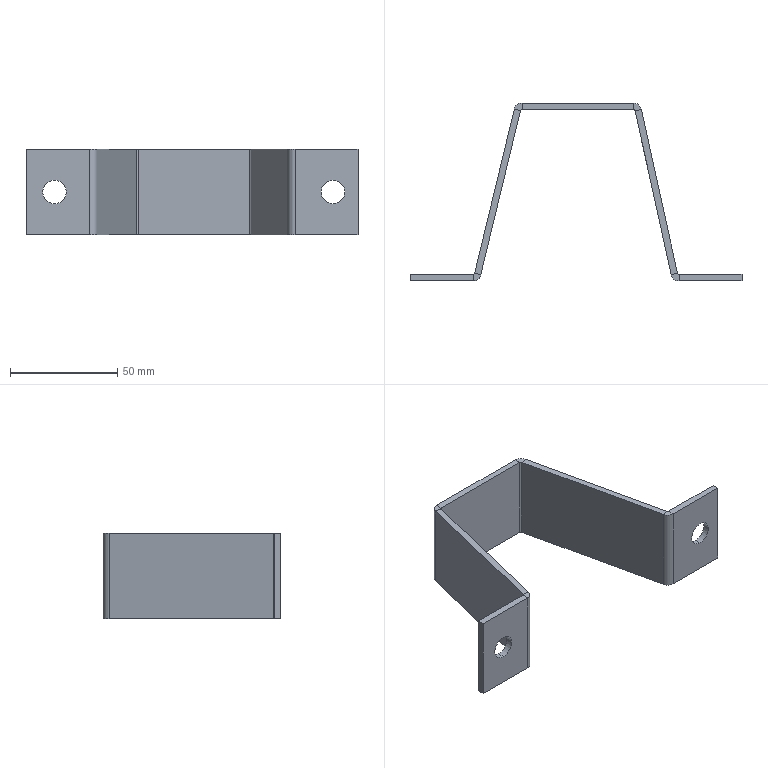Part | SolidWorks | features FlatPattern 1, ICE 1, SMBaseFlange 1, SheetMetal 1 | 1 solid | 42 faces | box 155 x 83 x 40 mm | volume 33033 mm3 | plane 30 | cylinder 12 | commonest cylinder face diameters 1.473 x4 7.473 x4 11 x4
STEP:
#1=CARTESIAN_POINT('',(73.722,-14.635,14.5));
#2=VERTEX_POINT('',#1);
#3=CARTESIAN_POINT('',(73.722,-14.635,25.5));
#4=VERTEX_POINT('',#3);
#5=CARTESIAN_POINT('',(73.722,-14.635,20.));
#6=DIRECTION('',(0.,1.,0.));
#7=DIRECTION('',(0.,0.,1.));
#8=AXIS2_PLACEMENT_3D('',#5,#6,#7);
#9=CIRCLE('',#8,5.5);
#10=EDGE_CURVE('',#2,#4,#9,.T.);
#11=ORIENTED_EDGE('',*,*,#10,.T.);
#12=CARTESIAN_POINT('',(73.722,-17.635,25.5));
#13=VERTEX_POINT('',#12);
#14=CARTESIAN_POINT('',(73.722,-7.635,25.5));
#15=DIRECTION('',(0.,-1.,0.));
#16=VECTOR('',#15,1000.);
#17=LINE('',#14,#16);
#18=EDGE_CURVE('',#4,#13,#17,.T.);
#19=ORIENTED_EDGE('',*,*,#18,.T.);
#20=CARTESIAN_POINT('',(73.722,-17.635,14.5));
#21=VERTEX_POINT('',#20);
#22=CARTESIAN_POINT('',(73.722,-17.635,20.));
#23=DIRECTION('',(0.,-1.,0.));
#24=DIRECTION('',(0.,0.,1.));
#25=AXIS2_PLACEMENT_3D('',#22,#23,#24);
#26=CIRCLE('',#25,5.5);
#27=EDGE_CURVE('',#13,#21,#26,.T.);
#28=ORIENTED_EDGE('',*,*,#27,.T.);
#29=CARTESIAN_POINT('',(73.722,-7.635,14.5));
#30=DIRECTION('',(0.,-1.,0.));
#31=VECTOR('',#30,1000.);
#32=LINE('',#29,#31);
#33=EDGE_CURVE('',#2,#21,#32,.T.);
#34=ORIENTED_EDGE('',*,*,#33,.F.);
#35=EDGE_LOOP('',(#11,#19,#28,#34));
#36=FACE_OUTER_BOUND('',#35,.T.);
#37=CARTESIAN_POINT('',(73.722,-7.635,20.));
#38=DIRECTION('',(0.,-1.,0.));
#39=DIRECTION('',(0.,0.,-1.));
#40=AXIS2_PLACEMENT_3D('',#37,#38,#39);
#41=CYLINDRICAL_SURFACE('',#40,5.5);
#42=ADVANCED_FACE('',(#36),#41,.F.);
#43=CARTESIAN_POINT('',(-56.278,-14.635,14.5));
#44=VERTEX_POINT('',#43);
#45=CARTESIAN_POINT('',(-56.278,-14.635,25.5));
#46=VERTEX_POINT('',#45);
#47=CARTESIAN_POINT('',(-56.278,-14.635,20.));
#48=DIRECTION('',(0.,1.,0.));
#49=DIRECTION('',(0.,0.,1.));
#50=AXIS2_PLACEMENT_3D('',#47,#48,#49);
#51=CIRCLE('',#50,5.5);
#52=EDGE_CURVE('',#44,#46,#51,.T.);
#53=ORIENTED_EDGE('',*,*,#52,.T.);
#54=CARTESIAN_POINT('',(-56.278,-17.635,25.5));
#55=VERTEX_POINT('',#54);
#56=CARTESIAN_POINT('',(-56.278,-7.635,25.5));
#57=DIRECTION('',(0.,-1.,0.));
#58=VECTOR('',#57,1000.);
#59=LINE('',#56,#58);
#60=EDGE_CURVE('',#46,#55,#59,.T.);
#61=ORIENTED_EDGE('',*,*,#60,.T.);
#62=CARTESIAN_POINT('',(-56.278,-17.635,14.5));
#63=VERTEX_POINT('',#62);
#64=CARTESIAN_POINT('',(-56.278,-17.635,20.));
#65=DIRECTION('',(0.,-1.,0.));
#66=DIRECTION('',(0.,0.,-1.));
#67=AXIS2_PLACEMENT_3D('',#64,#65,#66);
#68=CIRCLE('',#67,5.5);
#69=EDGE_CURVE('',#55,#63,#68,.T.);
#70=ORIENTED_EDGE('',*,*,#69,.T.);
#71=CARTESIAN_POINT('',(-56.278,-7.635,14.5));
#72=DIRECTION('',(0.,-1.,0.));
#73=VECTOR('',#72,1000.);
#74=LINE('',#71,#73);
#75=EDGE_CURVE('',#44,#63,#74,.T.);
#76=ORIENTED_EDGE('',*,*,#75,.F.);
#77=EDGE_LOOP('',(#53,#61,#70,#76));
#78=FACE_OUTER_BOUND('',#77,.T.);
#79=CARTESIAN_POINT('',(-56.278,-7.635,20.));
#80=DIRECTION('',(0.,-1.,0.));
#81=DIRECTION('',(0.,0.,-1.));
#82=AXIS2_PLACEMENT_3D('',#79,#80,#81);
#83=CYLINDRICAL_SURFACE('',#82,5.5);
#84=ADVANCED_FACE('',(#78),#83,.F.);
#85=CARTESIAN_POINT('',(-39.477,-14.072,40.));
#86=VERTEX_POINT('',#85);
#87=CARTESIAN_POINT('',(-36.561,-14.777,40.));
#88=VERTEX_POINT('',#87);
#89=CARTESIAN_POINT('',(-39.477,-14.072,40.));
#90=DIRECTION('',(0.9719,-0.2353,0.));
#91=VECTOR('',#90,1000.);
#92=LINE('',#89,#91);
#93=EDGE_CURVE('',#86,#88,#92,.T.);
#94=ORIENTED_EDGE('',*,*,#93,.F.);
#95=CARTESIAN_POINT('',(-40.193,-14.635,40.));
#96=VERTEX_POINT('',#95);
#97=CARTESIAN_POINT('',(-40.193,-13.898,40.));
#98=DIRECTION('',(0.,0.,1.));
#99=DIRECTION('',(-1.,0.,0.));
#100=AXIS2_PLACEMENT_3D('',#97,#98,#99);
#101=CIRCLE('',#100,0.7366);
#102=EDGE_CURVE('',#96,#86,#101,.T.);
#103=ORIENTED_EDGE('',*,*,#102,.F.);
#104=CARTESIAN_POINT('',(-40.193,-17.635,40.));
#105=VERTEX_POINT('',#104);
#106=CARTESIAN_POINT('',(-40.193,-17.635,40.));
#107=DIRECTION('',(0.,1.,0.));
#108=VECTOR('',#107,1000.);
#109=LINE('',#106,#108);
#110=EDGE_CURVE('',#105,#96,#109,.T.);
#111=ORIENTED_EDGE('',*,*,#110,.F.);
#112=CARTESIAN_POINT('',(-40.193,-13.898,40.));
#113=DIRECTION('',(0.,0.,1.));
#114=DIRECTION('',(1.,0.,0.));
#115=AXIS2_PLACEMENT_3D('',#112,#113,#114);
#116=CIRCLE('',#115,3.737);
#117=EDGE_CURVE('',#105,#88,#116,.T.);
#118=ORIENTED_EDGE('',*,*,#117,.T.);
#119=EDGE_LOOP('',(#94,#103,#111,#118));
#120=FACE_OUTER_BOUND('',#119,.T.);
#121=CARTESIAN_POINT('',(-39.477,-14.072,40.));
#122=DIRECTION('',(0.,0.,1.));
#123=DIRECTION('',(1.,0.,0.));
#124=AXIS2_PLACEMENT_3D('',#121,#122,#123);
#125=PLANE('',#124);
#126=ADVANCED_FACE('',(#120),#125,.T.);
#127=CARTESIAN_POINT('',(-20.938,62.508,40.));
#128=VERTEX_POINT('',#127);
#129=CARTESIAN_POINT('',(-39.613,-14.635,40.));
#130=DIRECTION('',(0.2353,0.9719,0.));
#131=VECTOR('',#130,1000.);
#132=LINE('',#129,#131);
#133=EDGE_CURVE('',#86,#128,#132,.T.);
#134=ORIENTED_EDGE('',*,*,#133,.F.);
#135=ORIENTED_EDGE('',*,*,#93,.T.);
#136=CARTESIAN_POINT('',(-18.023,61.802,40.));
#137=VERTEX_POINT('',#136);
#138=CARTESIAN_POINT('',(-36.697,-15.341,40.));
#139=DIRECTION('',(0.2353,0.9719,0.));
#140=VECTOR('',#139,1000.);
#141=LINE('',#138,#140);
#142=EDGE_CURVE('',#88,#137,#141,.T.);
#143=ORIENTED_EDGE('',*,*,#142,.T.);
#144=CARTESIAN_POINT('',(-18.023,61.802,40.));
#145=DIRECTION('',(-0.9719,0.2353,0.));
#146=VECTOR('',#145,1000.);
#147=LINE('',#144,#146);
#148=EDGE_CURVE('',#137,#128,#147,.T.);
#149=ORIENTED_EDGE('',*,*,#148,.T.);
#150=EDGE_LOOP('',(#134,#135,#143,#149));
#151=FACE_OUTER_BOUND('',#150,.T.);
#152=CARTESIAN_POINT('',(-40.193,-17.635,40.));
#153=DIRECTION('',(0.,0.,1.));
#154=DIRECTION('',(1.,0.,0.));
#155=AXIS2_PLACEMENT_3D('',#152,#153,#154);
#156=PLANE('',#155);
#157=ADVANCED_FACE('',(#151),#156,.T.);
#158=CARTESIAN_POINT('',(-40.193,-14.635,0.));
#159=VERTEX_POINT('',#158);
#160=CARTESIAN_POINT('',(-40.193,-17.635,0.));
#161=VERTEX_POINT('',#160);
#162=CARTESIAN_POINT('',(-40.193,-14.635,0.));
#163=DIRECTION('',(0.,-1.,0.));
#164=VECTOR('',#163,1000.);
#165=LINE('',#162,#164);
#166=EDGE_CURVE('',#159,#161,#165,.T.);
#167=ORIENTED_EDGE('',*,*,#166,.F.);
#168=CARTESIAN_POINT('',(-39.477,-14.072,0.));
#169=VERTEX_POINT('',#168);
#170=CARTESIAN_POINT('',(-40.193,-13.898,0.));
#171=DIRECTION('',(0.,0.,1.));
#172=DIRECTION('',(-1.,0.,0.));
#173=AXIS2_PLACEMENT_3D('',#170,#171,#172);
#174=CIRCLE('',#173,0.7366);
#175=EDGE_CURVE('',#159,#169,#174,.T.);
#176=ORIENTED_EDGE('',*,*,#175,.T.);
#177=CARTESIAN_POINT('',(-36.561,-14.777,0.));
#178=VERTEX_POINT('',#177);
#179=CARTESIAN_POINT('',(-36.561,-14.777,0.));
#180=DIRECTION('',(-0.9719,0.2353,0.));
#181=VECTOR('',#180,1000.);
#182=LINE('',#179,#181);
#183=EDGE_CURVE('',#178,#169,#182,.T.);
#184=ORIENTED_EDGE('',*,*,#183,.F.);
#185=CARTESIAN_POINT('',(-40.193,-13.898,0.));
#186=DIRECTION('',(0.,0.,1.));
#187=DIRECTION('',(1.,0.,0.));
#188=AXIS2_PLACEMENT_3D('',#185,#186,#187);
#189=CIRCLE('',#188,3.737);
#190=EDGE_CURVE('',#161,#178,#189,.T.);
#191=ORIENTED_EDGE('',*,*,#190,.F.);
#192=EDGE_LOOP('',(#167,#176,#184,#191));
#193=FACE_OUTER_BOUND('',#192,.T.);
#194=CARTESIAN_POINT('',(-40.193,-14.635,0.));
#195=DIRECTION('',(0.,0.,-1.));
#196=DIRECTION('',(-1.,0.,0.));
#197=AXIS2_PLACEMENT_3D('',#194,#195,#196);
#198=PLANE('',#197);
#199=ADVANCED_FACE('',(#193),#198,.T.);
#200=CARTESIAN_POINT('',(-69.613,-14.635,0.));
#201=VERTEX_POINT('',#200);
#202=CARTESIAN_POINT('',(-69.613,-14.635,0.));
#203=DIRECTION('',(1.,0.,0.));
#204=VECTOR('',#203,1000.);
#205=LINE('',#202,#204);
#206=EDGE_CURVE('',#201,#159,#205,.T.);
#207=ORIENTED_EDGE('',*,*,#206,.T.);
#208=ORIENTED_EDGE('',*,*,#166,.T.);
#209=CARTESIAN_POINT('',(-69.613,-17.635,0.));
#210=VERTEX_POINT('',#209);
#211=CARTESIAN_POINT('',(-69.613,-17.635,0.));
#212=DIRECTION('',(1.,0.,0.));
#213=VECTOR('',#212,1000.);
#214=LINE('',#211,#213);
#215=EDGE_CURVE('',#210,#161,#214,.T.);
#216=ORIENTED_EDGE('',*,*,#215,.F.);
#217=CARTESIAN_POINT('',(-69.613,-17.635,0.));
#218=DIRECTION('',(0.,1.,0.));
#219=VECTOR('',#218,1000.);
#220=LINE('',#217,#219);
#221=EDGE_CURVE('',#210,#201,#220,.T.);
#222=ORIENTED_EDGE('',*,*,#221,.T.);
#223=EDGE_LOOP('',(#207,#208,#216,#222));
#224=FACE_OUTER_BOUND('',#223,.T.);
#225=CARTESIAN_POINT('',(-36.561,-14.777,0.));
#226=DIRECTION('',(0.,0.,-1.));
#227=DIRECTION('',(-1.,0.,0.));
#228=AXIS2_PLACEMENT_3D('',#225,#226,#227);
#229=PLANE('',#228);
#230=ADVANCED_FACE('',(#224),#229,.T.);
#231=CARTESIAN_POINT('',(-17.307,65.365,40.));
#232=VERTEX_POINT('',#231);
#233=CARTESIAN_POINT('',(-17.307,62.365,40.));
#234=VERTEX_POINT('',#233);
#235=CARTESIAN_POINT('',(-17.307,65.365,40.));
#236=DIRECTION('',(0.,-1.,0.));
#237=VECTOR('',#236,1000.);
#238=LINE('',#235,#237);
#239=EDGE_CURVE('',#232,#234,#238,.T.);
#240=ORIENTED_EDGE('',*,*,#239,.F.);
#241=CARTESIAN_POINT('',(-17.307,61.629,40.));
#242=DIRECTION('',(0.,0.,-1.));
#243=DIRECTION('',(1.,0.,0.));
#244=AXIS2_PLACEMENT_3D('',#241,#242,#243);
#245=CIRCLE('',#244,3.737);
#246=EDGE_CURVE('',#128,#232,#245,.T.);
#247=ORIENTED_EDGE('',*,*,#246,.F.);
#248=ORIENTED_EDGE('',*,*,#148,.F.);
#249=CARTESIAN_POINT('',(-17.307,61.629,40.));
#250=DIRECTION('',(0.,0.,-1.));
#251=DIRECTION('',(1.,0.,0.));
#252=AXIS2_PLACEMENT_3D('',#249,#250,#251);
#253=CIRCLE('',#252,0.7366);
#254=EDGE_CURVE('',#137,#234,#253,.T.);
#255=ORIENTED_EDGE('',*,*,#254,.T.);
#256=EDGE_LOOP('',(#240,#247,#248,#255));
#257=FACE_OUTER_BOUND('',#256,.T.);
#258=CARTESIAN_POINT('',(-17.307,65.365,40.));
#259=DIRECTION('',(0.,0.,1.));
#260=DIRECTION('',(1.,0.,0.));
#261=AXIS2_PLACEMENT_3D('',#258,#259,#260);
#262=PLANE('',#261);
#263=ADVANCED_FACE('',(#257),#262,.T.);
#264=CARTESIAN_POINT('',(34.751,65.365,40.));
#265=VERTEX_POINT('',#264);
#266=CARTESIAN_POINT('',(-20.247,65.365,40.));
#267=DIRECTION('',(1.,0.,0.));
#268=VECTOR('',#267,1000.);
#269=LINE('',#266,#268);
#270=EDGE_CURVE('',#232,#265,#269,.T.);
#271=ORIENTED_EDGE('',*,*,#270,.F.);
#272=ORIENTED_EDGE('',*,*,#239,.T.);
#273=CARTESIAN_POINT('',(34.751,62.365,40.));
#274=VERTEX_POINT('',#273);
#275=CARTESIAN_POINT('',(-20.247,62.365,40.));
#276=DIRECTION('',(1.,0.,0.));
#277=VECTOR('',#276,1000.);
#278=LINE('',#275,#277);
#279=EDGE_CURVE('',#234,#274,#278,.T.);
#280=ORIENTED_EDGE('',*,*,#279,.T.);
#281=CARTESIAN_POINT('',(34.751,62.365,40.));
#282=DIRECTION('',(0.,1.,0.));
#283=VECTOR('',#282,1000.);
#284=LINE('',#281,#283);
#285=EDGE_CURVE('',#274,#265,#284,.T.);
#286=ORIENTED_EDGE('',*,*,#285,.T.);
#287=EDGE_LOOP('',(#271,#272,#280,#286));
#288=FACE_OUTER_BOUND('',#287,.T.);
#289=CARTESIAN_POINT('',(-18.023,61.802,40.));
#290=DIRECTION('',(0.,0.,1.));
#291=DIRECTION('',(1.,0.,0.));
#292=AXIS2_PLACEMENT_3D('',#289,#290,#291);
#293=PLANE('',#292);
#294=ADVANCED_FACE('',(#288),#293,.T.);
#295=CARTESIAN_POINT('',(-20.938,62.508,0.));
#296=VERTEX_POINT('',#295);
#297=CARTESIAN_POINT('',(-18.023,61.802,0.));
#298=VERTEX_POINT('',#297);
#299=CARTESIAN_POINT('',(-20.938,62.508,0.));
#300=DIRECTION('',(0.9719,-0.2353,0.));
#301=VECTOR('',#300,1000.);
#302=LINE('',#299,#301);
#303=EDGE_CURVE('',#296,#298,#302,.T.);
#304=ORIENTED_EDGE('',*,*,#303,.F.);
#305=CARTESIAN_POINT('',(-17.307,65.365,0.));
#306=VERTEX_POINT('',#305);
#307=CARTESIAN_POINT('',(-17.307,61.629,0.));
#308=DIRECTION('',(0.,0.,-1.));
#309=DIRECTION('',(1.,0.,0.));
#310=AXIS2_PLACEMENT_3D('',#307,#308,#309);
#311=CIRCLE('',#310,3.737);
#312=EDGE_CURVE('',#296,#306,#311,.T.);
#313=ORIENTED_EDGE('',*,*,#312,.T.);
#314=CARTESIAN_POINT('',(-17.307,62.365,0.));
#315=VERTEX_POINT('',#314);
#316=CARTESIAN_POINT('',(-17.307,62.365,0.));
#317=DIRECTION('',(0.,1.,0.));
#318=VECTOR('',#317,1000.);
#319=LINE('',#316,#318);
#320=EDGE_CURVE('',#315,#306,#319,.T.);
#321=ORIENTED_EDGE('',*,*,#320,.F.);
#322=CARTESIAN_POINT('',(-17.307,61.629,0.));
#323=DIRECTION('',(0.,0.,-1.));
#324=DIRECTION('',(1.,0.,0.));
#325=AXIS2_PLACEMENT_3D('',#322,#323,#324);
#326=CIRCLE('',#325,0.7366);
#327=EDGE_CURVE('',#298,#315,#326,.T.);
#328=ORIENTED_EDGE('',*,*,#327,.F.);
#329=EDGE_LOOP('',(#304,#313,#321,#328));
#330=FACE_OUTER_BOUND('',#329,.T.);
#331=CARTESIAN_POINT('',(-20.938,62.508,0.));
#332=DIRECTION('',(0.,0.,-1.));
#333=DIRECTION('',(-1.,0.,0.));
#334=AXIS2_PLACEMENT_3D('',#331,#332,#333);
#335=PLANE('',#334);
#336=ADVANCED_FACE('',(#330),#335,.T.);
#337=CARTESIAN_POINT('',(-39.613,-14.635,0.));
#338=DIRECTION('',(0.2353,0.9719,0.));
#339=VECTOR('',#338,1000.);
#340=LINE('',#337,#339);
#341=EDGE_CURVE('',#169,#296,#340,.T.);
#342=ORIENTED_EDGE('',*,*,#341,.T.);
#343=ORIENTED_EDGE('',*,*,#303,.T.);
#344=CARTESIAN_POINT('',(-36.697,-15.341,0.));
#345=DIRECTION('',(0.2353,0.9719,0.));
#346=VECTOR('',#345,1000.);
#347=LINE('',#344,#346);
#348=EDGE_CURVE('',#178,#298,#347,.T.);
#349=ORIENTED_EDGE('',*,*,#348,.F.);
#350=ORIENTED_EDGE('',*,*,#183,.T.);
#351=EDGE_LOOP('',(#342,#343,#349,#350));
#352=FACE_OUTER_BOUND('',#351,.T.);
#353=CARTESIAN_POINT('',(-17.307,62.365,0.));
#354=DIRECTION('',(0.,0.,-1.));
#355=DIRECTION('',(-1.,0.,0.));
#356=AXIS2_PLACEMENT_3D('',#353,#354,#355);
#357=PLANE('',#356);
#358=ADVANCED_FACE('',(#352),#357,.T.);
#359=CARTESIAN_POINT('',(38.4,62.433,40.));
#360=VERTEX_POINT('',#359);
#361=CARTESIAN_POINT('',(35.47,61.787,40.));
#362=VERTEX_POINT('',#361);
#363=CARTESIAN_POINT('',(38.4,62.433,40.));
#364=DIRECTION('',(-0.9766,-0.2153,0.));
#365=VECTOR('',#364,1000.);
#366=LINE('',#363,#365);
#367=EDGE_CURVE('',#360,#362,#366,.T.);
#368=ORIENTED_EDGE('',*,*,#367,.F.);
#369=CARTESIAN_POINT('',(34.751,61.629,40.));
#370=DIRECTION('',(0.,0.,-1.));
#371=DIRECTION('',(1.,0.,0.));
#372=AXIS2_PLACEMENT_3D('',#369,#370,#371);
#373=CIRCLE('',#372,3.737);
#374=EDGE_CURVE('',#265,#360,#373,.T.);
#375=ORIENTED_EDGE('',*,*,#374,.F.);
#376=ORIENTED_EDGE('',*,*,#285,.F.);
#377=CARTESIAN_POINT('',(34.751,61.629,40.));
#378=DIRECTION('',(0.,0.,-1.));
#379=DIRECTION('',(1.,0.,0.));
#380=AXIS2_PLACEMENT_3D('',#377,#378,#379);
#381=CIRCLE('',#380,0.7366);
#382=EDGE_CURVE('',#274,#362,#381,.T.);
#383=ORIENTED_EDGE('',*,*,#382,.T.);
#384=EDGE_LOOP('',(#368,#375,#376,#383));
#385=FACE_OUTER_BOUND('',#384,.T.);
#386=CARTESIAN_POINT('',(38.4,62.433,40.));
#387=DIRECTION('',(0.,0.,1.));
#388=DIRECTION('',(1.,0.,0.));
#389=AXIS2_PLACEMENT_3D('',#386,#387,#388);
#390=PLANE('',#389);
#391=ADVANCED_FACE('',(#385),#390,.T.);
#392=CARTESIAN_POINT('',(55.259,-14.057,40.));
#393=VERTEX_POINT('',#392);
#394=CARTESIAN_POINT('',(37.753,65.365,40.));
#395=DIRECTION('',(0.2153,-0.9766,0.));
#396=VECTOR('',#395,1000.);
#397=LINE('',#394,#396);
#398=EDGE_CURVE('',#360,#393,#397,.T.);
#399=ORIENTED_EDGE('',*,*,#398,.F.);
#400=ORIENTED_EDGE('',*,*,#367,.T.);
#401=CARTESIAN_POINT('',(52.33,-14.703,40.));
#402=VERTEX_POINT('',#401);
#403=CARTESIAN_POINT('',(34.824,64.719,40.));
#404=DIRECTION('',(0.2153,-0.9766,0.));
#405=VECTOR('',#404,1000.);
#406=LINE('',#403,#405);
#407=EDGE_CURVE('',#362,#402,#406,.T.);
#408=ORIENTED_EDGE('',*,*,#407,.T.);
#409=CARTESIAN_POINT('',(52.33,-14.703,40.));
#410=DIRECTION('',(0.9766,0.2153,0.));
#411=VECTOR('',#410,1000.);
#412=LINE('',#409,#411);
#413=EDGE_CURVE('',#402,#393,#412,.T.);
#414=ORIENTED_EDGE('',*,*,#413,.T.);
#415=EDGE_LOOP('',(#399,#400,#408,#414));
#416=FACE_OUTER_BOUND('',#415,.T.);
#417=CARTESIAN_POINT('',(34.751,62.365,40.));
#418=DIRECTION('',(0.,0.,1.));
#419=DIRECTION('',(1.,0.,0.));
#420=AXIS2_PLACEMENT_3D('',#417,#418,#419);
#421=PLANE('',#420);
#422=ADVANCED_FACE('',(#416),#421,.T.);
#423=CARTESIAN_POINT('',(34.751,65.365,0.));
#424=VERTEX_POINT('',#423);
#425=CARTESIAN_POINT('',(34.751,62.365,0.));
#426=VERTEX_POINT('',#425);
#427=CARTESIAN_POINT('',(34.751,65.365,0.));
#428=DIRECTION('',(0.,-1.,0.));
#429=VECTOR('',#428,1000.);
#430=LINE('',#427,#429);
#431=EDGE_CURVE('',#424,#426,#430,.T.);
#432=ORIENTED_EDGE('',*,*,#431,.F.);
#433=CARTESIAN_POINT('',(38.4,62.433,0.));
#434=VERTEX_POINT('',#433);
#435=CARTESIAN_POINT('',(34.751,61.629,0.));
#436=DIRECTION('',(0.,0.,-1.));
#437=DIRECTION('',(1.,0.,0.));
#438=AXIS2_PLACEMENT_3D('',#435,#436,#437);
#439=CIRCLE('',#438,3.737);
#440=EDGE_CURVE('',#424,#434,#439,.T.);
#441=ORIENTED_EDGE('',*,*,#440,.T.);
#442=CARTESIAN_POINT('',(35.47,61.787,0.));
#443=VERTEX_POINT('',#442);
#444=CARTESIAN_POINT('',(35.47,61.787,0.));
#445=DIRECTION('',(0.9766,0.2153,0.));
#446=VECTOR('',#445,1000.);
#447=LINE('',#444,#446);
#448=EDGE_CURVE('',#443,#434,#447,.T.);
#449=ORIENTED_EDGE('',*,*,#448,.F.);
#450=CARTESIAN_POINT('',(34.751,61.629,0.));
#451=DIRECTION('',(0.,0.,-1.));
#452=DIRECTION('',(1.,0.,0.));
#453=AXIS2_PLACEMENT_3D('',#450,#451,#452);
#454=CIRCLE('',#453,0.7366);
#455=EDGE_CURVE('',#426,#443,#454,.T.);
#456=ORIENTED_EDGE('',*,*,#455,.F.);
#457=EDGE_LOOP('',(#432,#441,#449,#456));
#458=FACE_OUTER_BOUND('',#457,.T.);
#459=CARTESIAN_POINT('',(34.751,65.365,0.));
#460=DIRECTION('',(0.,0.,-1.));
#461=DIRECTION('',(-1.,0.,0.));
#462=AXIS2_PLACEMENT_3D('',#459,#460,#461);
#463=PLANE('',#462);
#464=ADVANCED_FACE('',(#458),#463,.T.);
#465=CARTESIAN_POINT('',(-20.247,65.365,0.));
#466=DIRECTION('',(1.,0.,0.));
#467=VECTOR('',#466,1000.);
#468=LINE('',#465,#467);
#469=EDGE_CURVE('',#306,#424,#468,.T.);
#470=ORIENTED_EDGE('',*,*,#469,.T.);
#471=ORIENTED_EDGE('',*,*,#431,.T.);
#472=CARTESIAN_POINT('',(-20.247,62.365,0.));
#473=DIRECTION('',(1.,0.,0.));
#474=VECTOR('',#473,1000.);
#475=LINE('',#472,#474);
#476=EDGE_CURVE('',#315,#426,#475,.T.);
#477=ORIENTED_EDGE('',*,*,#476,.F.);
#478=ORIENTED_EDGE('',*,*,#320,.T.);
#479=EDGE_LOOP('',(#470,#471,#477,#478));
#480=FACE_OUTER_BOUND('',#479,.T.);
#481=CARTESIAN_POINT('',(35.47,61.787,0.));
#482=DIRECTION('',(0.,0.,-1.));
#483=DIRECTION('',(-1.,0.,0.));
#484=AXIS2_PLACEMENT_3D('',#481,#482,#483);
#485=PLANE('',#484);
#486=ADVANCED_FACE('',(#480),#485,.T.);
#487=CARTESIAN_POINT('',(55.979,-14.635,40.));
#488=VERTEX_POINT('',#487);
#489=CARTESIAN_POINT('',(55.979,-17.635,40.));
#490=VERTEX_POINT('',#489);
#491=CARTESIAN_POINT('',(55.979,-14.635,40.));
#492=DIRECTION('',(0.,-1.,0.));
#493=VECTOR('',#492,1000.);
#494=LINE('',#491,#493);
#495=EDGE_CURVE('',#488,#490,#494,.T.);
#496=ORIENTED_EDGE('',*,*,#495,.F.);
#497=CARTESIAN_POINT('',(55.979,-13.898,40.));
#498=DIRECTION('',(0.,0.,1.));
#499=DIRECTION('',(-1.,0.,0.));
#500=AXIS2_PLACEMENT_3D('',#497,#498,#499);
#501=CIRCLE('',#500,0.7366);
#502=EDGE_CURVE('',#393,#488,#501,.T.);
#503=ORIENTED_EDGE('',*,*,#502,.F.);
#504=ORIENTED_EDGE('',*,*,#413,.F.);
#505=CARTESIAN_POINT('',(55.979,-13.898,40.));
#506=DIRECTION('',(0.,0.,1.));
#507=DIRECTION('',(1.,0.,0.));
#508=AXIS2_PLACEMENT_3D('',#505,#506,#507);
#509=CIRCLE('',#508,3.737);
#510=EDGE_CURVE('',#402,#490,#509,.T.);
#511=ORIENTED_EDGE('',*,*,#510,.T.);
#512=EDGE_LOOP('',(#496,#503,#504,#511));
#513=FACE_OUTER_BOUND('',#512,.T.);
#514=CARTESIAN_POINT('',(55.979,-14.635,40.));
#515=DIRECTION('',(0.,0.,1.));
#516=DIRECTION('',(1.,0.,0.));
#517=AXIS2_PLACEMENT_3D('',#514,#515,#516);
#518=PLANE('',#517);
#519=ADVANCED_FACE('',(#513),#518,.T.);
#520=CARTESIAN_POINT('',(85.387,-14.635,40.));
#521=VERTEX_POINT('',#520);
#522=CARTESIAN_POINT('',(55.387,-14.635,40.));
#523=DIRECTION('',(1.,0.,0.));
#524=VECTOR('',#523,1000.);
#525=LINE('',#522,#524);
#526=EDGE_CURVE('',#488,#521,#525,.T.);
#527=ORIENTED_EDGE('',*,*,#526,.F.);
#528=ORIENTED_EDGE('',*,*,#495,.T.);
#529=CARTESIAN_POINT('',(85.387,-17.635,40.));
#530=VERTEX_POINT('',#529);
#531=CARTESIAN_POINT('',(55.387,-17.635,40.));
#532=DIRECTION('',(1.,0.,0.));
#533=VECTOR('',#532,1000.);
#534=LINE('',#531,#533);
#535=EDGE_CURVE('',#490,#530,#534,.T.);
#536=ORIENTED_EDGE('',*,*,#535,.T.);
#537=CARTESIAN_POINT('',(85.387,-14.635,40.));
#538=DIRECTION('',(0.,-1.,0.));
#539=VECTOR('',#538,1000.);
#540=LINE('',#537,#539);
#541=EDGE_CURVE('',#521,#530,#540,.T.);
#542=ORIENTED_EDGE('',*,*,#541,.F.);
#543=EDGE_LOOP('',(#527,#528,#536,#542));
#544=FACE_OUTER_BOUND('',#543,.T.);
#545=CARTESIAN_POINT('',(52.33,-14.703,40.));
#546=DIRECTION('',(0.,0.,1.));
#547=DIRECTION('',(1.,0.,0.));
#548=AXIS2_PLACEMENT_3D('',#545,#546,#547);
#549=PLANE('',#548);
#550=ADVANCED_FACE('',(#544),#549,.T.);
#551=CARTESIAN_POINT('',(55.259,-14.057,0.));
#552=VERTEX_POINT('',#551);
#553=CARTESIAN_POINT('',(52.33,-14.703,0.));
#554=VERTEX_POINT('',#553);
#555=CARTESIAN_POINT('',(55.259,-14.057,0.));
#556=DIRECTION('',(-0.9766,-0.2153,0.));
#557=VECTOR('',#556,1000.);
#558=LINE('',#555,#557);
#559=EDGE_CURVE('',#552,#554,#558,.T.);
#560=ORIENTED_EDGE('',*,*,#559,.F.);
#561=CARTESIAN_POINT('',(55.979,-14.635,0.));
#562=VERTEX_POINT('',#561);
#563=CARTESIAN_POINT('',(55.979,-13.898,0.));
#564=DIRECTION('',(0.,0.,1.));
#565=DIRECTION('',(-1.,0.,0.));
#566=AXIS2_PLACEMENT_3D('',#563,#564,#565);
#567=CIRCLE('',#566,0.7366);
#568=EDGE_CURVE('',#552,#562,#567,.T.);
#569=ORIENTED_EDGE('',*,*,#568,.T.);
#570=CARTESIAN_POINT('',(55.979,-17.635,0.));
#571=VERTEX_POINT('',#570);
#572=CARTESIAN_POINT('',(55.979,-17.635,0.));
#573=DIRECTION('',(0.,1.,0.));
#574=VECTOR('',#573,1000.);
#575=LINE('',#572,#574);
#576=EDGE_CURVE('',#571,#562,#575,.T.);
#577=ORIENTED_EDGE('',*,*,#576,.F.);
#578=CARTESIAN_POINT('',(55.979,-13.898,0.));
#579=DIRECTION('',(0.,0.,1.));
#580=DIRECTION('',(1.,0.,0.));
#581=AXIS2_PLACEMENT_3D('',#578,#579,#580);
#582=CIRCLE('',#581,3.737);
#583=EDGE_CURVE('',#554,#571,#582,.T.);
#584=ORIENTED_EDGE('',*,*,#583,.F.);
#585=EDGE_LOOP('',(#560,#569,#577,#584));
#586=FACE_OUTER_BOUND('',#585,.T.);
#587=CARTESIAN_POINT('',(55.259,-14.057,0.));
#588=DIRECTION('',(0.,0.,-1.));
#589=DIRECTION('',(-1.,0.,0.));
#590=AXIS2_PLACEMENT_3D('',#587,#588,#589);
#591=PLANE('',#590);
#592=ADVANCED_FACE('',(#586),#591,.T.);
#593=CARTESIAN_POINT('',(37.753,65.365,0.));
#594=DIRECTION('',(0.2153,-0.9766,0.));
#595=VECTOR('',#594,1000.);
#596=LINE('',#593,#595);
#597=EDGE_CURVE('',#434,#552,#596,.T.);
#598=ORIENTED_EDGE('',*,*,#597,.T.);
#599=ORIENTED_EDGE('',*,*,#559,.T.);
#600=CARTESIAN_POINT('',(34.824,64.719,0.));
#601=DIRECTION('',(0.2153,-0.9766,0.));
#602=VECTOR('',#601,1000.);
#603=LINE('',#600,#602);
#604=EDGE_CURVE('',#443,#554,#603,.T.);
#605=ORIENTED_EDGE('',*,*,#604,.F.);
#606=ORIENTED_EDGE('',*,*,#448,.T.);
#607=EDGE_LOOP('',(#598,#599,#605,#606));
#608=FACE_OUTER_BOUND('',#607,.T.);
#609=CARTESIAN_POINT('',(55.979,-17.635,0.));
#610=DIRECTION('',(0.,0.,-1.));
#611=DIRECTION('',(-1.,0.,0.));
#612=AXIS2_PLACEMENT_3D('',#609,#610,#611);
#613=PLANE('',#612);
#614=ADVANCED_FACE('',(#608),#613,.T.);
#615=CARTESIAN_POINT('',(73.722,-17.635,20.));
#616=DIRECTION('',(0.,-1.,0.));
#617=DIRECTION('',(0.,0.,1.));
#618=AXIS2_PLACEMENT_3D('',#615,#616,#617);
#619=CIRCLE('',#618,5.5);
#620=EDGE_CURVE('',#21,#13,#619,.T.);
#621=ORIENTED_EDGE('',*,*,#620,.F.);
#622=ORIENTED_EDGE('',*,*,#27,.F.);
#623=EDGE_LOOP('',(#621,#622));
#624=FACE_BOUND('',#623,.T.);
#625=CARTESIAN_POINT('',(85.387,-17.635,0.));
#626=VERTEX_POINT('',#625);
#627=CARTESIAN_POINT('',(55.387,-17.635,0.));
#628=DIRECTION('',(1.,0.,0.));
#629=VECTOR('',#628,1000.);
#630=LINE('',#627,#629);
#631=EDGE_CURVE('',#571,#626,#630,.T.);
#632=ORIENTED_EDGE('',*,*,#631,.T.);
#633=CARTESIAN_POINT('',(85.387,-17.635,40.));
#634=DIRECTION('',(0.,0.,-1.));
#635=VECTOR('',#634,1000.);
#636=LINE('',#633,#635);
#637=EDGE_CURVE('',#530,#626,#636,.T.);
#638=ORIENTED_EDGE('',*,*,#637,.F.);
#639=ORIENTED_EDGE('',*,*,#535,.F.);
#640=CARTESIAN_POINT('',(55.979,-17.635,40.));
#641=DIRECTION('',(0.,0.,-1.));
#642=VECTOR('',#641,1000.);
#643=LINE('',#640,#642);
#644=EDGE_CURVE('',#490,#571,#643,.T.);
#645=ORIENTED_EDGE('',*,*,#644,.T.);
#646=EDGE_LOOP('',(#632,#638,#639,#645));
#647=FACE_OUTER_BOUND('',#646,.T.);
#648=CARTESIAN_POINT('',(55.387,-17.635,40.));
#649=DIRECTION('',(0.,1.,0.));
#650=DIRECTION('',(0.,0.,1.));
#651=AXIS2_PLACEMENT_3D('',#648,#649,#650);
#652=PLANE('',#651);
#653=ADVANCED_FACE('',(#624,#647),#652,.F.);
#654=CARTESIAN_POINT('',(85.387,-14.635,0.));
#655=VERTEX_POINT('',#654);
#656=CARTESIAN_POINT('',(85.387,-14.635,0.));
#657=DIRECTION('',(0.,-1.,0.));
#658=VECTOR('',#657,1000.);
#659=LINE('',#656,#658);
#660=EDGE_CURVE('',#655,#626,#659,.T.);
#661=ORIENTED_EDGE('',*,*,#660,.F.);
#662=CARTESIAN_POINT('',(85.387,-14.635,40.));
#663=DIRECTION('',(0.,0.,-1.));
#664=VECTOR('',#663,1000.);
#665=LINE('',#662,#664);
#666=EDGE_CURVE('',#521,#655,#665,.T.);
#667=ORIENTED_EDGE('',*,*,#666,.F.);
#668=ORIENTED_EDGE('',*,*,#541,.T.);
#669=ORIENTED_EDGE('',*,*,#637,.T.);
#670=EDGE_LOOP('',(#661,#667,#668,#669));
#671=FACE_OUTER_BOUND('',#670,.T.);
#672=CARTESIAN_POINT('',(85.387,-14.635,40.));
#673=DIRECTION('',(1.,0.,0.));
#674=DIRECTION('',(0.,0.,-1.));
#675=AXIS2_PLACEMENT_3D('',#672,#673,#674);
#676=PLANE('',#675);
#677=ADVANCED_FACE('',(#671),#676,.T.);
#678=ORIENTED_EDGE('',*,*,#10,.F.);
#679=CARTESIAN_POINT('',(73.722,-14.635,20.));
#680=DIRECTION('',(0.,1.,0.));
#681=DIRECTION('',(0.,0.,1.));
#682=AXIS2_PLACEMENT_3D('',#679,#680,#681);
#683=CIRCLE('',#682,5.5);
#684=EDGE_CURVE('',#4,#2,#683,.T.);
#685=ORIENTED_EDGE('',*,*,#684,.F.);
#686=EDGE_LOOP('',(#678,#685));
#687=FACE_BOUND('',#686,.T.);
#688=CARTESIAN_POINT('',(55.387,-14.635,0.));
#689=DIRECTION('',(1.,0.,0.));
#690=VECTOR('',#689,1000.);
#691=LINE('',#688,#690);
#692=EDGE_CURVE('',#562,#655,#691,.T.);
#693=ORIENTED_EDGE('',*,*,#692,.F.);
#694=CARTESIAN_POINT('',(55.979,-14.635,40.));
#695=DIRECTION('',(0.,0.,-1.));
#696=VECTOR('',#695,1000.);
#697=LINE('',#694,#696);
#698=EDGE_CURVE('',#488,#562,#697,.T.);
#699=ORIENTED_EDGE('',*,*,#698,.F.);
#700=ORIENTED_EDGE('',*,*,#526,.T.);
#701=ORIENTED_EDGE('',*,*,#666,.T.);
#702=EDGE_LOOP('',(#693,#699,#700,#701));
#703=FACE_OUTER_BOUND('',#702,.T.);
#704=CARTESIAN_POINT('',(55.387,-14.635,40.));
#705=DIRECTION('',(0.,1.,0.));
#706=DIRECTION('',(0.,0.,1.));
#707=AXIS2_PLACEMENT_3D('',#704,#705,#706);
#708=PLANE('',#707);
#709=ADVANCED_FACE('',(#687,#703),#708,.T.);
#710=ORIENTED_EDGE('',*,*,#568,.F.);
#711=CARTESIAN_POINT('',(55.259,-14.057,40.));
#712=DIRECTION('',(0.,0.,-1.));
#713=VECTOR('',#712,1000.);
#714=LINE('',#711,#713);
#715=EDGE_CURVE('',#393,#552,#714,.T.);
#716=ORIENTED_EDGE('',*,*,#715,.F.);
#717=ORIENTED_EDGE('',*,*,#502,.T.);
#718=ORIENTED_EDGE('',*,*,#698,.T.);
#719=EDGE_LOOP('',(#710,#716,#717,#718));
#720=FACE_OUTER_BOUND('',#719,.T.);
#721=CARTESIAN_POINT('',(55.979,-13.898,40.));
#722=DIRECTION('',(0.,0.,-1.));
#723=DIRECTION('',(-1.,0.,0.));
#724=AXIS2_PLACEMENT_3D('',#721,#722,#723);
#725=CYLINDRICAL_SURFACE('',#724,0.7366);
#726=ADVANCED_FACE('',(#720),#725,.F.);
#727=ORIENTED_EDGE('',*,*,#597,.F.);
#728=CARTESIAN_POINT('',(38.4,62.433,40.));
#729=DIRECTION('',(0.,0.,-1.));
#730=VECTOR('',#729,1000.);
#731=LINE('',#728,#730);
#732=EDGE_CURVE('',#360,#434,#731,.T.);
#733=ORIENTED_EDGE('',*,*,#732,.F.);
#734=ORIENTED_EDGE('',*,*,#398,.T.);
#735=ORIENTED_EDGE('',*,*,#715,.T.);
#736=EDGE_LOOP('',(#727,#733,#734,#735));
#737=FACE_OUTER_BOUND('',#736,.T.);
#738=CARTESIAN_POINT('',(37.753,65.365,40.));
#739=DIRECTION('',(0.9766,0.2153,0.));
#740=DIRECTION('',(-0.2153,0.9766,0.));
#741=AXIS2_PLACEMENT_3D('',#738,#739,#740);
#742=PLANE('',#741);
#743=ADVANCED_FACE('',(#737),#742,.T.);
#744=ORIENTED_EDGE('',*,*,#440,.F.);
#745=CARTESIAN_POINT('',(34.751,65.365,40.));
#746=DIRECTION('',(0.,0.,-1.));
#747=VECTOR('',#746,1000.);
#748=LINE('',#745,#747);
#749=EDGE_CURVE('',#265,#424,#748,.T.);
#750=ORIENTED_EDGE('',*,*,#749,.F.);
#751=ORIENTED_EDGE('',*,*,#374,.T.);
#752=ORIENTED_EDGE('',*,*,#732,.T.);
#753=EDGE_LOOP('',(#744,#750,#751,#752));
#754=FACE_OUTER_BOUND('',#753,.T.);
#755=CARTESIAN_POINT('',(34.751,61.629,40.));
#756=DIRECTION('',(0.,0.,-1.));
#757=DIRECTION('',(-1.,0.,0.));
#758=AXIS2_PLACEMENT_3D('',#755,#756,#757);
#759=CYLINDRICAL_SURFACE('',#758,3.737);
#760=ADVANCED_FACE('',(#754),#759,.T.);
#761=ORIENTED_EDGE('',*,*,#469,.F.);
#762=CARTESIAN_POINT('',(-17.307,65.365,40.));
#763=DIRECTION('',(0.,0.,-1.));
#764=VECTOR('',#763,1000.);
#765=LINE('',#762,#764);
#766=EDGE_CURVE('',#232,#306,#765,.T.);
#767=ORIENTED_EDGE('',*,*,#766,.F.);
#768=ORIENTED_EDGE('',*,*,#270,.T.);
#769=ORIENTED_EDGE('',*,*,#749,.T.);
#770=EDGE_LOOP('',(#761,#767,#768,#769));
#771=FACE_OUTER_BOUND('',#770,.T.);
#772=CARTESIAN_POINT('',(-20.247,65.365,40.));
#773=DIRECTION('',(0.,1.,0.));
#774=DIRECTION('',(0.,0.,1.));
#775=AXIS2_PLACEMENT_3D('',#772,#773,#774);
#776=PLANE('',#775);
#777=ADVANCED_FACE('',(#771),#776,.T.);
#778=ORIENTED_EDGE('',*,*,#312,.F.);
#779=CARTESIAN_POINT('',(-20.938,62.508,40.));
#780=DIRECTION('',(0.,0.,-1.));
#781=VECTOR('',#780,1000.);
#782=LINE('',#779,#781);
#783=EDGE_CURVE('',#128,#296,#782,.T.);
#784=ORIENTED_EDGE('',*,*,#783,.F.);
#785=ORIENTED_EDGE('',*,*,#246,.T.);
#786=ORIENTED_EDGE('',*,*,#766,.T.);
#787=EDGE_LOOP('',(#778,#784,#785,#786));
#788=FACE_OUTER_BOUND('',#787,.T.);
#789=CARTESIAN_POINT('',(-17.307,61.629,40.));
#790=DIRECTION('',(0.,0.,-1.));
#791=DIRECTION('',(-1.,0.,0.));
#792=AXIS2_PLACEMENT_3D('',#789,#790,#791);
#793=CYLINDRICAL_SURFACE('',#792,3.737);
#794=ADVANCED_FACE('',(#788),#793,.T.);
#795=ORIENTED_EDGE('',*,*,#341,.F.);
#796=CARTESIAN_POINT('',(-39.477,-14.072,40.));
#797=DIRECTION('',(0.,0.,-1.));
#798=VECTOR('',#797,1000.);
#799=LINE('',#796,#798);
#800=EDGE_CURVE('',#86,#169,#799,.T.);
#801=ORIENTED_EDGE('',*,*,#800,.F.);
#802=ORIENTED_EDGE('',*,*,#133,.T.);
#803=ORIENTED_EDGE('',*,*,#783,.T.);
#804=EDGE_LOOP('',(#795,#801,#802,#803));
#805=FACE_OUTER_BOUND('',#804,.T.);
#806=CARTESIAN_POINT('',(-39.613,-14.635,40.));
#807=DIRECTION('',(-0.9719,0.2353,0.));
#808=DIRECTION('',(-0.2353,-0.9719,0.));
#809=AXIS2_PLACEMENT_3D('',#806,#807,#808);
#810=PLANE('',#809);
#811=ADVANCED_FACE('',(#805),#810,.T.);
#812=ORIENTED_EDGE('',*,*,#175,.F.);
#813=CARTESIAN_POINT('',(-40.193,-14.635,40.));
#814=DIRECTION('',(0.,0.,-1.));
#815=VECTOR('',#814,1000.);
#816=LINE('',#813,#815);
#817=EDGE_CURVE('',#96,#159,#816,.T.);
#818=ORIENTED_EDGE('',*,*,#817,.F.);
#819=ORIENTED_EDGE('',*,*,#102,.T.);
#820=ORIENTED_EDGE('',*,*,#800,.T.);
#821=EDGE_LOOP('',(#812,#818,#819,#820));
#822=FACE_OUTER_BOUND('',#821,.T.);
#823=CARTESIAN_POINT('',(-40.193,-13.898,40.));
#824=DIRECTION('',(0.,0.,-1.));
#825=DIRECTION('',(-1.,0.,0.));
#826=AXIS2_PLACEMENT_3D('',#823,#824,#825);
#827=CYLINDRICAL_SURFACE('',#826,0.7366);
#828=ADVANCED_FACE('',(#822),#827,.F.);
#829=ORIENTED_EDGE('',*,*,#52,.F.);
#830=CARTESIAN_POINT('',(-56.278,-14.635,20.));
#831=DIRECTION('',(0.,1.,0.));
#832=DIRECTION('',(0.,0.,1.));
#833=AXIS2_PLACEMENT_3D('',#830,#831,#832);
#834=CIRCLE('',#833,5.5);
#835=EDGE_CURVE('',#46,#44,#834,.T.);
#836=ORIENTED_EDGE('',*,*,#835,.F.);
#837=EDGE_LOOP('',(#829,#836));
#838=FACE_BOUND('',#837,.T.);
#839=ORIENTED_EDGE('',*,*,#206,.F.);
#840=CARTESIAN_POINT('',(-69.613,-14.635,40.));
#841=VERTEX_POINT('',#840);
#842=CARTESIAN_POINT('',(-69.613,-14.635,40.));
#843=DIRECTION('',(0.,0.,-1.));
#844=VECTOR('',#843,1000.);
#845=LINE('',#842,#844);
#846=EDGE_CURVE('',#841,#201,#845,.T.);
#847=ORIENTED_EDGE('',*,*,#846,.F.);
#848=CARTESIAN_POINT('',(-69.613,-14.635,40.));
#849=DIRECTION('',(1.,0.,0.));
#850=VECTOR('',#849,1000.);
#851=LINE('',#848,#850);
#852=EDGE_CURVE('',#841,#96,#851,.T.);
#853=ORIENTED_EDGE('',*,*,#852,.T.);
#854=ORIENTED_EDGE('',*,*,#817,.T.);
#855=EDGE_LOOP('',(#839,#847,#853,#854));
#856=FACE_OUTER_BOUND('',#855,.T.);
#857=CARTESIAN_POINT('',(-69.613,-14.635,40.));
#858=DIRECTION('',(0.,1.,0.));
#859=DIRECTION('',(0.,0.,1.));
#860=AXIS2_PLACEMENT_3D('',#857,#858,#859);
#861=PLANE('',#860);
#862=ADVANCED_FACE('',(#838,#856),#861,.T.);
#863=ORIENTED_EDGE('',*,*,#221,.F.);
#864=CARTESIAN_POINT('',(-69.613,-17.635,40.));
#865=VERTEX_POINT('',#864);
#866=CARTESIAN_POINT('',(-69.613,-17.635,40.));
#867=DIRECTION('',(0.,0.,-1.));
#868=VECTOR('',#867,1000.);
#869=LINE('',#866,#868);
#870=EDGE_CURVE('',#865,#210,#869,.T.);
#871=ORIENTED_EDGE('',*,*,#870,.F.);
#872=CARTESIAN_POINT('',(-69.613,-17.635,40.));
#873=DIRECTION('',(0.,1.,0.));
#874=VECTOR('',#873,1000.);
#875=LINE('',#872,#874);
#876=EDGE_CURVE('',#865,#841,#875,.T.);
#877=ORIENTED_EDGE('',*,*,#876,.T.);
#878=ORIENTED_EDGE('',*,*,#846,.T.);
#879=EDGE_LOOP('',(#863,#871,#877,#878));
#880=FACE_OUTER_BOUND('',#879,.T.);
#881=CARTESIAN_POINT('',(-69.613,-17.635,40.));
#882=DIRECTION('',(-1.,0.,0.));
#883=DIRECTION('',(0.,0.,1.));
#884=AXIS2_PLACEMENT_3D('',#881,#882,#883);
#885=PLANE('',#884);
#886=ADVANCED_FACE('',(#880),#885,.T.);
#887=CARTESIAN_POINT('',(-56.278,-17.635,20.));
#888=DIRECTION('',(0.,-1.,0.));
#889=DIRECTION('',(0.,0.,-1.));
#890=AXIS2_PLACEMENT_3D('',#887,#888,#889);
#891=CIRCLE('',#890,5.5);
#892=EDGE_CURVE('',#63,#55,#891,.T.);
#893=ORIENTED_EDGE('',*,*,#892,.F.);
#894=ORIENTED_EDGE('',*,*,#69,.F.);
#895=EDGE_LOOP('',(#893,#894));
#896=FACE_BOUND('',#895,.T.);
#897=ORIENTED_EDGE('',*,*,#215,.T.);
#898=CARTESIAN_POINT('',(-40.193,-17.635,40.));
#899=DIRECTION('',(0.,0.,-1.));
#900=VECTOR('',#899,1000.);
#901=LINE('',#898,#900);
#902=EDGE_CURVE('',#105,#161,#901,.T.);
#903=ORIENTED_EDGE('',*,*,#902,.F.);
#904=CARTESIAN_POINT('',(-69.613,-17.635,40.));
#905=DIRECTION('',(1.,0.,0.));
#906=VECTOR('',#905,1000.);
#907=LINE('',#904,#906);
#908=EDGE_CURVE('',#865,#105,#907,.T.);
#909=ORIENTED_EDGE('',*,*,#908,.F.);
#910=ORIENTED_EDGE('',*,*,#870,.T.);
#911=EDGE_LOOP('',(#897,#903,#909,#910));
#912=FACE_OUTER_BOUND('',#911,.T.);
#913=CARTESIAN_POINT('',(-69.613,-17.635,40.));
#914=DIRECTION('',(0.,1.,0.));
#915=DIRECTION('',(0.,0.,1.));
#916=AXIS2_PLACEMENT_3D('',#913,#914,#915);
#917=PLANE('',#916);
#918=ADVANCED_FACE('',(#896,#912),#917,.F.);
#919=ORIENTED_EDGE('',*,*,#190,.T.);
#920=CARTESIAN_POINT('',(-36.561,-14.777,40.));
#921=DIRECTION('',(0.,0.,-1.));
#922=VECTOR('',#921,1000.);
#923=LINE('',#920,#922);
#924=EDGE_CURVE('',#88,#178,#923,.T.);
#925=ORIENTED_EDGE('',*,*,#924,.F.);
#926=ORIENTED_EDGE('',*,*,#117,.F.);
#927=ORIENTED_EDGE('',*,*,#902,.T.);
#928=EDGE_LOOP('',(#919,#925,#926,#927));
#929=FACE_OUTER_BOUND('',#928,.T.);
#930=CARTESIAN_POINT('',(-40.193,-13.898,40.));
#931=DIRECTION('',(0.,0.,-1.));
#932=DIRECTION('',(-1.,0.,0.));
#933=AXIS2_PLACEMENT_3D('',#930,#931,#932);
#934=CYLINDRICAL_SURFACE('',#933,3.737);
#935=ADVANCED_FACE('',(#929),#934,.T.);
#936=ORIENTED_EDGE('',*,*,#348,.T.);
#937=CARTESIAN_POINT('',(-18.023,61.802,40.));
#938=DIRECTION('',(0.,0.,-1.));
#939=VECTOR('',#938,1000.);
#940=LINE('',#937,#939);
#941=EDGE_CURVE('',#137,#298,#940,.T.);
#942=ORIENTED_EDGE('',*,*,#941,.F.);
#943=ORIENTED_EDGE('',*,*,#142,.F.);
#944=ORIENTED_EDGE('',*,*,#924,.T.);
#945=EDGE_LOOP('',(#936,#942,#943,#944));
#946=FACE_OUTER_BOUND('',#945,.T.);
#947=CARTESIAN_POINT('',(-36.697,-15.341,40.));
#948=DIRECTION('',(-0.9719,0.2353,0.));
#949=DIRECTION('',(-0.2353,-0.9719,0.));
#950=AXIS2_PLACEMENT_3D('',#947,#948,#949);
#951=PLANE('',#950);
#952=ADVANCED_FACE('',(#946),#951,.F.);
#953=ORIENTED_EDGE('',*,*,#327,.T.);
#954=CARTESIAN_POINT('',(-17.307,62.365,40.));
#955=DIRECTION('',(0.,0.,-1.));
#956=VECTOR('',#955,1000.);
#957=LINE('',#954,#956);
#958=EDGE_CURVE('',#234,#315,#957,.T.);
#959=ORIENTED_EDGE('',*,*,#958,.F.);
#960=ORIENTED_EDGE('',*,*,#254,.F.);
#961=ORIENTED_EDGE('',*,*,#941,.T.);
#962=EDGE_LOOP('',(#953,#959,#960,#961));
#963=FACE_OUTER_BOUND('',#962,.T.);
#964=CARTESIAN_POINT('',(-17.307,61.629,40.));
#965=DIRECTION('',(0.,0.,-1.));
#966=DIRECTION('',(-1.,0.,0.));
#967=AXIS2_PLACEMENT_3D('',#964,#965,#966);
#968=CYLINDRICAL_SURFACE('',#967,0.7366);
#969=ADVANCED_FACE('',(#963),#968,.F.);
#970=ORIENTED_EDGE('',*,*,#476,.T.);
#971=CARTESIAN_POINT('',(34.751,62.365,40.));
#972=DIRECTION('',(0.,0.,-1.));
#973=VECTOR('',#972,1000.);
#974=LINE('',#971,#973);
#975=EDGE_CURVE('',#274,#426,#974,.T.);
#976=ORIENTED_EDGE('',*,*,#975,.F.);
#977=ORIENTED_EDGE('',*,*,#279,.F.);
#978=ORIENTED_EDGE('',*,*,#958,.T.);
#979=EDGE_LOOP('',(#970,#976,#977,#978));
#980=FACE_OUTER_BOUND('',#979,.T.);
#981=CARTESIAN_POINT('',(-20.247,62.365,40.));
#982=DIRECTION('',(0.,1.,0.));
#983=DIRECTION('',(0.,0.,1.));
#984=AXIS2_PLACEMENT_3D('',#981,#982,#983);
#985=PLANE('',#984);
#986=ADVANCED_FACE('',(#980),#985,.F.);
#987=ORIENTED_EDGE('',*,*,#455,.T.);
#988=CARTESIAN_POINT('',(35.47,61.787,40.));
#989=DIRECTION('',(0.,0.,-1.));
#990=VECTOR('',#989,1000.);
#991=LINE('',#988,#990);
#992=EDGE_CURVE('',#362,#443,#991,.T.);
#993=ORIENTED_EDGE('',*,*,#992,.F.);
#994=ORIENTED_EDGE('',*,*,#382,.F.);
#995=ORIENTED_EDGE('',*,*,#975,.T.);
#996=EDGE_LOOP('',(#987,#993,#994,#995));
#997=FACE_OUTER_BOUND('',#996,.T.);
#998=CARTESIAN_POINT('',(34.751,61.629,40.));
#999=DIRECTION('',(0.,0.,-1.));
#1000=DIRECTION('',(-1.,0.,0.));
#1001=AXIS2_PLACEMENT_3D('',#998,#999,#1000);
#1002=CYLINDRICAL_SURFACE('',#1001,0.7366);
#1003=ADVANCED_FACE('',(#997),#1002,.F.);
#1004=ORIENTED_EDGE('',*,*,#604,.T.);
#1005=CARTESIAN_POINT('',(52.33,-14.703,40.));
#1006=DIRECTION('',(0.,0.,-1.));
#1007=VECTOR('',#1006,1000.);
#1008=LINE('',#1005,#1007);
#1009=EDGE_CURVE('',#402,#554,#1008,.T.);
#1010=ORIENTED_EDGE('',*,*,#1009,.F.);
#1011=ORIENTED_EDGE('',*,*,#407,.F.);
#1012=ORIENTED_EDGE('',*,*,#992,.T.);
#1013=EDGE_LOOP('',(#1004,#1010,#1011,#1012));
#1014=FACE_OUTER_BOUND('',#1013,.T.);
#1015=CARTESIAN_POINT('',(34.824,64.719,40.));
#1016=DIRECTION('',(0.9766,0.2153,0.));
#1017=DIRECTION('',(-0.2153,0.9766,0.));
#1018=AXIS2_PLACEMENT_3D('',#1015,#1016,#1017);
#1019=PLANE('',#1018);
#1020=ADVANCED_FACE('',(#1014),#1019,.F.);
#1021=ORIENTED_EDGE('',*,*,#583,.T.);
#1022=ORIENTED_EDGE('',*,*,#644,.F.);
#1023=ORIENTED_EDGE('',*,*,#510,.F.);
#1024=ORIENTED_EDGE('',*,*,#1009,.T.);
#1025=EDGE_LOOP('',(#1021,#1022,#1023,#1024));
#1026=FACE_OUTER_BOUND('',#1025,.T.);
#1027=CARTESIAN_POINT('',(55.979,-13.898,40.));
#1028=DIRECTION('',(0.,0.,-1.));
#1029=DIRECTION('',(-1.,0.,0.));
#1030=AXIS2_PLACEMENT_3D('',#1027,#1028,#1029);
#1031=CYLINDRICAL_SURFACE('',#1030,3.737);
#1032=ADVANCED_FACE('',(#1026),#1031,.T.);
#1033=ORIENTED_EDGE('',*,*,#908,.T.);
#1034=ORIENTED_EDGE('',*,*,#110,.T.);
#1035=ORIENTED_EDGE('',*,*,#852,.F.);
#1036=ORIENTED_EDGE('',*,*,#876,.F.);
#1037=EDGE_LOOP('',(#1033,#1034,#1035,#1036));
#1038=FACE_OUTER_BOUND('',#1037,.T.);
#1039=CARTESIAN_POINT('',(55.979,-13.898,40.));
#1040=DIRECTION('',(0.,0.,-1.));
#1041=DIRECTION('',(-1.,0.,0.));
#1042=AXIS2_PLACEMENT_3D('',#1039,#1040,#1041);
#1043=PLANE('',#1042);
#1044=ADVANCED_FACE('',(#1038),#1043,.F.);
#1045=ORIENTED_EDGE('',*,*,#631,.F.);
#1046=ORIENTED_EDGE('',*,*,#576,.T.);
#1047=ORIENTED_EDGE('',*,*,#692,.T.);
#1048=ORIENTED_EDGE('',*,*,#660,.T.);
#1049=EDGE_LOOP('',(#1045,#1046,#1047,#1048));
#1050=FACE_OUTER_BOUND('',#1049,.T.);
#1051=CARTESIAN_POINT('',(55.979,-13.898,0.));
#1052=DIRECTION('',(0.,0.,-1.));
#1053=DIRECTION('',(-1.,0.,0.));
#1054=AXIS2_PLACEMENT_3D('',#1051,#1052,#1053);
#1055=PLANE('',#1054);
#1056=ADVANCED_FACE('',(#1050),#1055,.T.);
#1057=ORIENTED_EDGE('',*,*,#60,.F.);
#1058=ORIENTED_EDGE('',*,*,#835,.T.);
#1059=ORIENTED_EDGE('',*,*,#75,.T.);
#1060=ORIENTED_EDGE('',*,*,#892,.T.);
#1061=EDGE_LOOP('',(#1057,#1058,#1059,#1060));
#1062=FACE_OUTER_BOUND('',#1061,.T.);
#1063=CARTESIAN_POINT('',(-56.278,-7.635,20.));
#1064=DIRECTION('',(0.,-1.,0.));
#1065=DIRECTION('',(0.,0.,-1.));
#1066=AXIS2_PLACEMENT_3D('',#1063,#1064,#1065);
#1067=CYLINDRICAL_SURFACE('',#1066,5.5);
#1068=ADVANCED_FACE('',(#1062),#1067,.F.);
#1069=ORIENTED_EDGE('',*,*,#18,.F.);
#1070=ORIENTED_EDGE('',*,*,#684,.T.);
#1071=ORIENTED_EDGE('',*,*,#33,.T.);
#1072=ORIENTED_EDGE('',*,*,#620,.T.);
#1073=EDGE_LOOP('',(#1069,#1070,#1071,#1072));
#1074=FACE_OUTER_BOUND('',#1073,.T.);
#1075=CARTESIAN_POINT('',(73.722,-7.635,20.));
#1076=DIRECTION('',(0.,-1.,0.));
#1077=DIRECTION('',(0.,0.,-1.));
#1078=AXIS2_PLACEMENT_3D('',#1075,#1076,#1077);
#1079=CYLINDRICAL_SURFACE('',#1078,5.5);
#1080=ADVANCED_FACE('',(#1074),#1079,.F.);
#1081=CLOSED_SHELL('',(#42,#84,#126,#157,#199,#230,#263,#294,#336,#358,#391,#422,#464,#486,#519,#550,#592,#614,#653,#677,#709,#726,#743,#760,#777,#794,#811,#828,#862,#886,#918,#935,#952,#969,#986,#1003,#1020,#1032,#1044,#1056,#1068,#1080));
#1082=MANIFOLD_SOLID_BREP('',#1081);
#1083=CARTESIAN_POINT('',(0.,0.,0.));
#1084=DIRECTION('',(0.,0.,1.));
#1085=DIRECTION('',(1.,0.,0.));
#1086=AXIS2_PLACEMENT_3D('',#1083,#1084,#1085);
#1087=(LENGTH_UNIT()NAMED_UNIT(*)SI_UNIT(.MILLI.,.METRE.));
#1088=UNCERTAINTY_MEASURE_WITH_UNIT(LENGTH_MEASURE(0.00001),#1087,'','');
#1089=(NAMED_UNIT(*)PLANE_ANGLE_UNIT()SI_UNIT($,.RADIAN.));
#1090=(NAMED_UNIT(*)SI_UNIT($,.STERADIAN.)SOLID_ANGLE_UNIT());
#1091=(GEOMETRIC_REPRESENTATION_CONTEXT(3)GLOBAL_UNCERTAINTY_ASSIGNED_CONTEXT((#1088))GLOBAL_UNIT_ASSIGNED_CONTEXT((#1087,#1089,#1090))REPRESENTATION_CONTEXT('',''));
#1092=ADVANCED_BREP_SHAPE_REPRESENTATION('',(#1082,#1086),#1091);